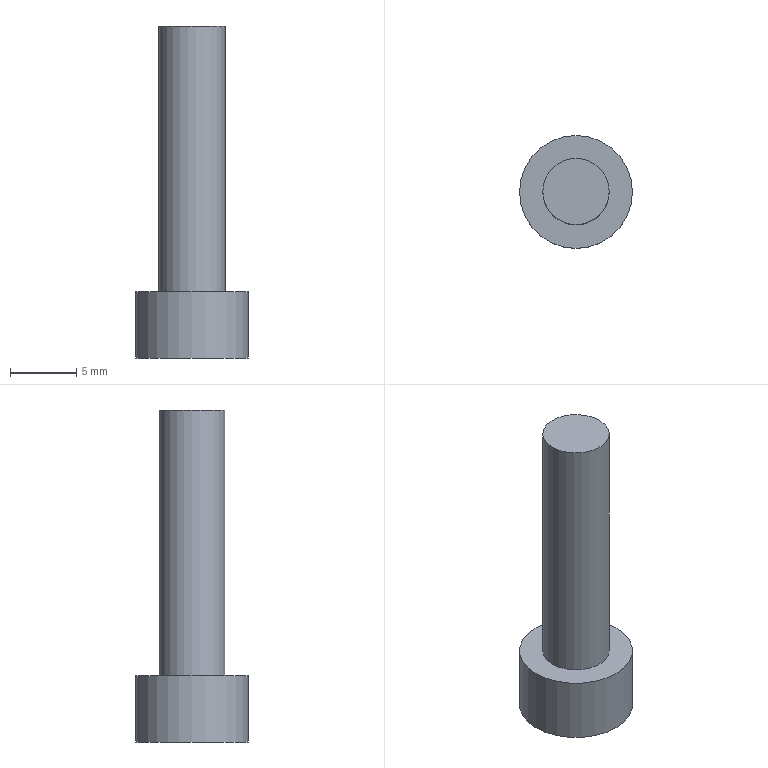Part | STEP file | 1 solid | 12 faces | box 8.5 x 8.5 x 25 mm | volume 630.698 mm3 | plane 10 | cylinder 2 | commonest cylinder face diameters 5 x1 8.5 x1
STEP:
#1=CARTESIAN_POINT('',(0.,0.,0.));
#2=DIRECTION('',(0.,0.,1.));
#3=DIRECTION('',(1.,0.,0.));
#4=AXIS2_PLACEMENT_3D('',#1,#2,#3);
#5=CARTESIAN_POINT('',(1537.233,391.98,-14.081));
#6=VERTEX_POINT('',#5);
#7=CARTESIAN_POINT('',(1541.483,391.98,-14.081));
#8=DIRECTION('',(0.,0.,-1.));
#9=DIRECTION('',(-1.,0.,0.));
#10=AXIS2_PLACEMENT_3D('',#7,#8,#9);
#11=CIRCLE('',#10,4.25);
#12=CARTESIAN_POINT('',(1537.233,391.98,-14.081));
#13=DIRECTION('',(0.,0.,1.));
#14=DIRECTION('',(1.,0.,0.));
#15=AXIS2_PLACEMENT_3D('',#12,#13,#14);
#16=PLANE('',#15);
#17=CARTESIAN_POINT('',(0.,0.));
#18=CARTESIAN_POINT('',(0.,7.361));
#19=CARTESIAN_POINT('',(6.375,3.681));
#20=CARTESIAN_POINT('',(12.75,0.));
#21=CARTESIAN_POINT('',(6.375,-3.681));
#22=CARTESIAN_POINT('',(0.,-7.361));
#23=CARTESIAN_POINT('',(0.,0.));
#24=(BOUNDED_CURVE()B_SPLINE_CURVE(2,(#17,#18,#19,#20,#21,#22,#23),.UNSPECIFIED.,.T.,.F.)B_SPLINE_CURVE_WITH_KNOTS((1,2,2,2,2,1),(-2.094,0.,2.094,4.189,6.283,8.378),.UNSPECIFIED.)CURVE()GEOMETRIC_REPRESENTATION_ITEM()RATIONAL_B_SPLINE_CURVE((1.,0.5,1.,0.5,1.,0.5,1.))REPRESENTATION_ITEM(''));
#25=(GEOMETRIC_REPRESENTATION_CONTEXT(2)PARAMETRIC_REPRESENTATION_CONTEXT()REPRESENTATION_CONTEXT('',''));
#26=DEFINITIONAL_REPRESENTATION('',(#24),#25);
#27=PCURVE('',#16,#26);
#28=CARTESIAN_POINT('',(1541.483,391.98,22.319));
#29=DIRECTION('',(0.,0.,-1.));
#30=DIRECTION('',(-1.,0.,0.));
#31=AXIS2_PLACEMENT_3D('',#28,#29,#30);
#32=CYLINDRICAL_SURFACE('',#31,4.25);
#33=CARTESIAN_POINT('',(0.,36.4));
#34=DIRECTION('',(1.,0.));
#35=VECTOR('',#34,1.);
#36=LINE('',#33,#35);
#37=(GEOMETRIC_REPRESENTATION_CONTEXT(2)PARAMETRIC_REPRESENTATION_CONTEXT()REPRESENTATION_CONTEXT('',''));
#38=DEFINITIONAL_REPRESENTATION('',(#36),#37);
#39=PCURVE('',#32,#38);
#40=SURFACE_CURVE('',#11,(#27,#39),.PCURVE_S1.);
#41=EDGE_CURVE('',#6,#6,#40,.T.);
#42=ORIENTED_EDGE('',*,*,#41,.T.);
#43=EDGE_LOOP('',(#42));
#44=FACE_BOUND('',#43,.T.);
#45=CARTESIAN_POINT('',(1542.638,393.98,-14.081));
#46=VERTEX_POINT('',#45);
#47=CARTESIAN_POINT('',(1540.328,393.98,-14.081));
#48=VERTEX_POINT('',#47);
#49=CARTESIAN_POINT('',(1542.638,393.98,-14.081));
#50=DIRECTION('',(-1.,0.,0.));
#51=VECTOR('',#50,1.);
#52=LINE('',#49,#51);
#53=CARTESIAN_POINT('',(5.405,2.));
#54=DIRECTION('',(-1.,0.));
#55=VECTOR('',#54,1.);
#56=LINE('',#53,#55);
#57=(GEOMETRIC_REPRESENTATION_CONTEXT(2)PARAMETRIC_REPRESENTATION_CONTEXT()REPRESENTATION_CONTEXT('',''));
#58=DEFINITIONAL_REPRESENTATION('',(#56),#57);
#59=PCURVE('',#16,#58);
#60=CARTESIAN_POINT('',(1542.638,393.98,-10.781));
#61=DIRECTION('',(0.,-1.,0.));
#62=DIRECTION('',(-1.,0.,0.));
#63=AXIS2_PLACEMENT_3D('',#60,#61,#62);
#64=PLANE('',#63);
#65=CARTESIAN_POINT('',(0.,3.3));
#66=DIRECTION('',(1.,0.));
#67=VECTOR('',#66,1.);
#68=LINE('',#65,#67);
#69=(GEOMETRIC_REPRESENTATION_CONTEXT(2)PARAMETRIC_REPRESENTATION_CONTEXT()REPRESENTATION_CONTEXT('',''));
#70=DEFINITIONAL_REPRESENTATION('',(#68),#69);
#71=PCURVE('',#64,#70);
#72=SURFACE_CURVE('',#52,(#59,#71),.PCURVE_S1.);
#73=EDGE_CURVE('',#46,#48,#72,.T.);
#74=ORIENTED_EDGE('',*,*,#73,.T.);
#75=CARTESIAN_POINT('',(1539.174,391.98,-14.081));
#76=VERTEX_POINT('',#75);
#77=CARTESIAN_POINT('',(1540.328,393.98,-14.081));
#78=DIRECTION('',(-0.5,-0.866,0.));
#79=VECTOR('',#78,1.);
#80=LINE('',#77,#79);
#81=CARTESIAN_POINT('',(3.095,2.));
#82=DIRECTION('',(-0.5,-0.866));
#83=VECTOR('',#82,1.);
#84=LINE('',#81,#83);
#85=(GEOMETRIC_REPRESENTATION_CONTEXT(2)PARAMETRIC_REPRESENTATION_CONTEXT()REPRESENTATION_CONTEXT('',''));
#86=DEFINITIONAL_REPRESENTATION('',(#84),#85);
#87=PCURVE('',#16,#86);
#88=CARTESIAN_POINT('',(1540.328,393.98,-10.781));
#89=DIRECTION('',(0.866,-0.5,0.));
#90=DIRECTION('',(-0.5,-0.866,0.));
#91=AXIS2_PLACEMENT_3D('',#88,#89,#90);
#92=PLANE('',#91);
#93=CARTESIAN_POINT('',(0.,3.3));
#94=DIRECTION('',(1.,0.));
#95=VECTOR('',#94,1.);
#96=LINE('',#93,#95);
#97=(GEOMETRIC_REPRESENTATION_CONTEXT(2)PARAMETRIC_REPRESENTATION_CONTEXT()REPRESENTATION_CONTEXT('',''));
#98=DEFINITIONAL_REPRESENTATION('',(#96),#97);
#99=PCURVE('',#92,#98);
#100=SURFACE_CURVE('',#80,(#87,#99),.PCURVE_S1.);
#101=EDGE_CURVE('',#48,#76,#100,.T.);
#102=ORIENTED_EDGE('',*,*,#101,.T.);
#103=CARTESIAN_POINT('',(1540.328,389.98,-14.081));
#104=VERTEX_POINT('',#103);
#105=CARTESIAN_POINT('',(1539.174,391.98,-14.081));
#106=DIRECTION('',(0.5,-0.866,0.));
#107=VECTOR('',#106,1.);
#108=LINE('',#105,#107);
#109=CARTESIAN_POINT('',(1.941,0.));
#110=DIRECTION('',(0.5,-0.866));
#111=VECTOR('',#110,1.);
#112=LINE('',#109,#111);
#113=(GEOMETRIC_REPRESENTATION_CONTEXT(2)PARAMETRIC_REPRESENTATION_CONTEXT()REPRESENTATION_CONTEXT('',''));
#114=DEFINITIONAL_REPRESENTATION('',(#112),#113);
#115=PCURVE('',#16,#114);
#116=CARTESIAN_POINT('',(1539.174,391.98,-10.781));
#117=DIRECTION('',(0.866,0.5,0.));
#118=DIRECTION('',(0.5,-0.866,0.));
#119=AXIS2_PLACEMENT_3D('',#116,#117,#118);
#120=PLANE('',#119);
#121=CARTESIAN_POINT('',(0.,3.3));
#122=DIRECTION('',(1.,0.));
#123=VECTOR('',#122,1.);
#124=LINE('',#121,#123);
#125=(GEOMETRIC_REPRESENTATION_CONTEXT(2)PARAMETRIC_REPRESENTATION_CONTEXT()REPRESENTATION_CONTEXT('',''));
#126=DEFINITIONAL_REPRESENTATION('',(#124),#125);
#127=PCURVE('',#120,#126);
#128=SURFACE_CURVE('',#108,(#115,#127),.PCURVE_S1.);
#129=EDGE_CURVE('',#76,#104,#128,.T.);
#130=ORIENTED_EDGE('',*,*,#129,.T.);
#131=CARTESIAN_POINT('',(1542.638,389.98,-14.081));
#132=VERTEX_POINT('',#131);
#133=CARTESIAN_POINT('',(1540.328,389.98,-14.081));
#134=DIRECTION('',(1.,0.,0.));
#135=VECTOR('',#134,1.);
#136=LINE('',#133,#135);
#137=CARTESIAN_POINT('',(3.095,-2.));
#138=DIRECTION('',(1.,0.));
#139=VECTOR('',#138,1.);
#140=LINE('',#137,#139);
#141=(GEOMETRIC_REPRESENTATION_CONTEXT(2)PARAMETRIC_REPRESENTATION_CONTEXT()REPRESENTATION_CONTEXT('',''));
#142=DEFINITIONAL_REPRESENTATION('',(#140),#141);
#143=PCURVE('',#16,#142);
#144=CARTESIAN_POINT('',(1540.328,389.98,-10.781));
#145=DIRECTION('',(0.,1.,0.));
#146=DIRECTION('',(0.,0.,-1.));
#147=AXIS2_PLACEMENT_3D('',#144,#145,#146);
#148=PLANE('',#147);
#149=CARTESIAN_POINT('',(3.3,0.));
#150=DIRECTION('',(0.,-1.));
#151=VECTOR('',#150,1.);
#152=LINE('',#149,#151);
#153=(GEOMETRIC_REPRESENTATION_CONTEXT(2)PARAMETRIC_REPRESENTATION_CONTEXT()REPRESENTATION_CONTEXT('',''));
#154=DEFINITIONAL_REPRESENTATION('',(#152),#153);
#155=PCURVE('',#148,#154);
#156=SURFACE_CURVE('',#136,(#143,#155),.PCURVE_S1.);
#157=EDGE_CURVE('',#104,#132,#156,.T.);
#158=ORIENTED_EDGE('',*,*,#157,.T.);
#159=CARTESIAN_POINT('',(1543.792,391.98,-14.081));
#160=VERTEX_POINT('',#159);
#161=CARTESIAN_POINT('',(1542.638,389.98,-14.081));
#162=DIRECTION('',(0.5,0.866,0.));
#163=VECTOR('',#162,1.);
#164=LINE('',#161,#163);
#165=CARTESIAN_POINT('',(5.405,-2.));
#166=DIRECTION('',(0.5,0.866));
#167=VECTOR('',#166,1.);
#168=LINE('',#165,#167);
#169=(GEOMETRIC_REPRESENTATION_CONTEXT(2)PARAMETRIC_REPRESENTATION_CONTEXT()REPRESENTATION_CONTEXT('',''));
#170=DEFINITIONAL_REPRESENTATION('',(#168),#169);
#171=PCURVE('',#16,#170);
#172=CARTESIAN_POINT('',(1542.638,389.98,-10.781));
#173=DIRECTION('',(-0.866,0.5,0.));
#174=DIRECTION('',(0.5,0.866,0.));
#175=AXIS2_PLACEMENT_3D('',#172,#173,#174);
#176=PLANE('',#175);
#177=CARTESIAN_POINT('',(0.,3.3));
#178=DIRECTION('',(1.,0.));
#179=VECTOR('',#178,1.);
#180=LINE('',#177,#179);
#181=(GEOMETRIC_REPRESENTATION_CONTEXT(2)PARAMETRIC_REPRESENTATION_CONTEXT()REPRESENTATION_CONTEXT('',''));
#182=DEFINITIONAL_REPRESENTATION('',(#180),#181);
#183=PCURVE('',#176,#182);
#184=SURFACE_CURVE('',#164,(#171,#183),.PCURVE_S1.);
#185=EDGE_CURVE('',#132,#160,#184,.T.);
#186=ORIENTED_EDGE('',*,*,#185,.T.);
#187=CARTESIAN_POINT('',(1543.792,391.98,-14.081));
#188=DIRECTION('',(-0.5,0.866,0.));
#189=VECTOR('',#188,1.);
#190=LINE('',#187,#189);
#191=CARTESIAN_POINT('',(6.559,0.));
#192=DIRECTION('',(-0.5,0.866));
#193=VECTOR('',#192,1.);
#194=LINE('',#191,#193);
#195=(GEOMETRIC_REPRESENTATION_CONTEXT(2)PARAMETRIC_REPRESENTATION_CONTEXT()REPRESENTATION_CONTEXT('',''));
#196=DEFINITIONAL_REPRESENTATION('',(#194),#195);
#197=PCURVE('',#16,#196);
#198=CARTESIAN_POINT('',(1543.792,391.98,-10.781));
#199=DIRECTION('',(-0.866,-0.5,0.));
#200=DIRECTION('',(-0.5,0.866,0.));
#201=AXIS2_PLACEMENT_3D('',#198,#199,#200);
#202=PLANE('',#201);
#203=CARTESIAN_POINT('',(0.,3.3));
#204=DIRECTION('',(1.,0.));
#205=VECTOR('',#204,1.);
#206=LINE('',#203,#205);
#207=(GEOMETRIC_REPRESENTATION_CONTEXT(2)PARAMETRIC_REPRESENTATION_CONTEXT()REPRESENTATION_CONTEXT('',''));
#208=DEFINITIONAL_REPRESENTATION('',(#206),#207);
#209=PCURVE('',#202,#208);
#210=SURFACE_CURVE('',#190,(#197,#209),.PCURVE_S1.);
#211=EDGE_CURVE('',#160,#46,#210,.T.);
#212=ORIENTED_EDGE('',*,*,#211,.T.);
#213=EDGE_LOOP('',(#74,#102,#130,#158,#186,#212));
#214=FACE_BOUND('',#213,.T.);
#215=ADVANCED_FACE('',(#44,#214),#16,.F.);
#216=ORIENTED_EDGE('',*,*,#41,.F.);
#217=CARTESIAN_POINT('',(1537.233,391.98,-9.081));
#218=VERTEX_POINT('',#217);
#219=CARTESIAN_POINT('',(1537.233,391.98,-9.081));
#220=CARTESIAN_POINT('',(1537.233,391.98,-14.081));
#221=B_SPLINE_CURVE_WITH_KNOTS('',1,(#219,#220),.UNSPECIFIED.,.F.,.F.,(2,2),(31.4,36.4),.PIECEWISE_BEZIER_KNOTS.);
#222=CARTESIAN_POINT('',(0.,0.));
#223=DIRECTION('',(0.,1.));
#224=VECTOR('',#223,1.);
#225=LINE('',#222,#224);
#226=(GEOMETRIC_REPRESENTATION_CONTEXT(2)PARAMETRIC_REPRESENTATION_CONTEXT()REPRESENTATION_CONTEXT('',''));
#227=DEFINITIONAL_REPRESENTATION('',(#225),#226);
#228=PCURVE('',#32,#227);
#229=CARTESIAN_POINT('',(6.283,0.));
#230=DIRECTION('',(0.,1.));
#231=VECTOR('',#230,1.);
#232=LINE('',#229,#231);
#233=(GEOMETRIC_REPRESENTATION_CONTEXT(2)PARAMETRIC_REPRESENTATION_CONTEXT()REPRESENTATION_CONTEXT('',''));
#234=DEFINITIONAL_REPRESENTATION('',(#232),#233);
#235=PCURVE('',#32,#234);
#236=SEAM_CURVE('',#221,(#228,#235),.PCURVE_S1.);
#237=EDGE_CURVE('',#218,#6,#236,.T.);
#238=ORIENTED_EDGE('',*,*,#237,.F.);
#239=CARTESIAN_POINT('',(1541.483,391.98,-9.081));
#240=DIRECTION('',(0.,0.,-1.));
#241=DIRECTION('',(-1.,0.,0.));
#242=AXIS2_PLACEMENT_3D('',#239,#240,#241);
#243=CIRCLE('',#242,4.25);
#244=CARTESIAN_POINT('',(0.,31.4));
#245=DIRECTION('',(1.,0.));
#246=VECTOR('',#245,1.);
#247=LINE('',#244,#246);
#248=(GEOMETRIC_REPRESENTATION_CONTEXT(2)PARAMETRIC_REPRESENTATION_CONTEXT()REPRESENTATION_CONTEXT('',''));
#249=DEFINITIONAL_REPRESENTATION('',(#247),#248);
#250=PCURVE('',#32,#249);
#251=CARTESIAN_POINT('',(1538.983,391.98,-9.081));
#252=DIRECTION('',(0.,0.,-1.));
#253=DIRECTION('',(-1.,0.,0.));
#254=AXIS2_PLACEMENT_3D('',#251,#252,#253);
#255=PLANE('',#254);
#256=CARTESIAN_POINT('',(-2.5,0.));
#257=DIRECTION('',(1.,0.));
#258=AXIS2_PLACEMENT_2D('',#256,#257);
#259=CIRCLE('',#258,4.25);
#260=(GEOMETRIC_REPRESENTATION_CONTEXT(2)PARAMETRIC_REPRESENTATION_CONTEXT()REPRESENTATION_CONTEXT('',''));
#261=DEFINITIONAL_REPRESENTATION('',(#259),#260);
#262=PCURVE('',#255,#261);
#263=SURFACE_CURVE('',#243,(#250,#262),.PCURVE_S1.);
#264=EDGE_CURVE('',#218,#218,#263,.T.);
#265=ORIENTED_EDGE('',*,*,#264,.T.);
#266=ORIENTED_EDGE('',*,*,#237,.T.);
#267=EDGE_LOOP('',(#216,#238,#265,#266));
#268=FACE_BOUND('',#267,.T.);
#269=ADVANCED_FACE('',(#268),#32,.T.);
#270=ORIENTED_EDGE('',*,*,#264,.F.);
#271=EDGE_LOOP('',(#270));
#272=FACE_BOUND('',#271,.T.);
#273=CARTESIAN_POINT('',(1538.983,391.98,-9.081));
#274=VERTEX_POINT('',#273);
#275=CARTESIAN_POINT('',(1541.483,391.98,-9.081));
#276=DIRECTION('',(0.,0.,-1.));
#277=DIRECTION('',(-1.,0.,0.));
#278=AXIS2_PLACEMENT_3D('',#275,#276,#277);
#279=CIRCLE('',#278,2.5);
#280=CARTESIAN_POINT('',(-2.5,0.));
#281=DIRECTION('',(1.,0.));
#282=AXIS2_PLACEMENT_2D('',#280,#281);
#283=CIRCLE('',#282,2.5);
#284=(GEOMETRIC_REPRESENTATION_CONTEXT(2)PARAMETRIC_REPRESENTATION_CONTEXT()REPRESENTATION_CONTEXT('',''));
#285=DEFINITIONAL_REPRESENTATION('',(#283),#284);
#286=PCURVE('',#255,#285);
#287=CARTESIAN_POINT('',(1541.483,391.98,22.319));
#288=DIRECTION('',(0.,0.,-1.));
#289=DIRECTION('',(-1.,0.,0.));
#290=AXIS2_PLACEMENT_3D('',#287,#288,#289);
#291=CYLINDRICAL_SURFACE('',#290,2.5);
#292=CARTESIAN_POINT('',(0.,31.4));
#293=DIRECTION('',(1.,0.));
#294=VECTOR('',#293,1.);
#295=LINE('',#292,#294);
#296=(GEOMETRIC_REPRESENTATION_CONTEXT(2)PARAMETRIC_REPRESENTATION_CONTEXT()REPRESENTATION_CONTEXT('',''));
#297=DEFINITIONAL_REPRESENTATION('',(#295),#296);
#298=PCURVE('',#291,#297);
#299=SURFACE_CURVE('',#279,(#286,#298),.PCURVE_S1.);
#300=EDGE_CURVE('',#274,#274,#299,.T.);
#301=ORIENTED_EDGE('',*,*,#300,.T.);
#302=EDGE_LOOP('',(#301));
#303=FACE_BOUND('',#302,.T.);
#304=ADVANCED_FACE('',(#272,#303),#255,.F.);
#305=ORIENTED_EDGE('',*,*,#300,.F.);
#306=CARTESIAN_POINT('',(1538.983,391.98,10.919));
#307=VERTEX_POINT('',#306);
#308=CARTESIAN_POINT('',(1538.983,391.98,10.919));
#309=CARTESIAN_POINT('',(1538.983,391.98,-9.081));
#310=B_SPLINE_CURVE_WITH_KNOTS('',1,(#308,#309),.UNSPECIFIED.,.F.,.F.,(2,2),(11.4,31.4),.PIECEWISE_BEZIER_KNOTS.);
#311=CARTESIAN_POINT('',(0.,0.));
#312=DIRECTION('',(0.,1.));
#313=VECTOR('',#312,1.);
#314=LINE('',#311,#313);
#315=(GEOMETRIC_REPRESENTATION_CONTEXT(2)PARAMETRIC_REPRESENTATION_CONTEXT()REPRESENTATION_CONTEXT('',''));
#316=DEFINITIONAL_REPRESENTATION('',(#314),#315);
#317=PCURVE('',#291,#316);
#318=CARTESIAN_POINT('',(6.283,0.));
#319=DIRECTION('',(0.,1.));
#320=VECTOR('',#319,1.);
#321=LINE('',#318,#320);
#322=(GEOMETRIC_REPRESENTATION_CONTEXT(2)PARAMETRIC_REPRESENTATION_CONTEXT()REPRESENTATION_CONTEXT('',''));
#323=DEFINITIONAL_REPRESENTATION('',(#321),#322);
#324=PCURVE('',#291,#323);
#325=SEAM_CURVE('',#310,(#317,#324),.PCURVE_S1.);
#326=EDGE_CURVE('',#307,#274,#325,.T.);
#327=ORIENTED_EDGE('',*,*,#326,.F.);
#328=CARTESIAN_POINT('',(1541.483,391.98,10.919));
#329=DIRECTION('',(0.,0.,-1.));
#330=DIRECTION('',(-1.,0.,0.));
#331=AXIS2_PLACEMENT_3D('',#328,#329,#330);
#332=CIRCLE('',#331,2.5);
#333=CARTESIAN_POINT('',(0.,11.4));
#334=DIRECTION('',(1.,0.));
#335=VECTOR('',#334,1.);
#336=LINE('',#333,#335);
#337=(GEOMETRIC_REPRESENTATION_CONTEXT(2)PARAMETRIC_REPRESENTATION_CONTEXT()REPRESENTATION_CONTEXT('',''));
#338=DEFINITIONAL_REPRESENTATION('',(#336),#337);
#339=PCURVE('',#291,#338);
#340=CARTESIAN_POINT('',(1541.483,391.98,10.919));
#341=DIRECTION('',(0.,0.,-1.));
#342=DIRECTION('',(-1.,0.,0.));
#343=AXIS2_PLACEMENT_3D('',#340,#341,#342);
#344=PLANE('',#343);
#345=CARTESIAN_POINT('',(0.,0.));
#346=DIRECTION('',(1.,0.));
#347=AXIS2_PLACEMENT_2D('',#345,#346);
#348=CIRCLE('',#347,2.5);
#349=(GEOMETRIC_REPRESENTATION_CONTEXT(2)PARAMETRIC_REPRESENTATION_CONTEXT()REPRESENTATION_CONTEXT('',''));
#350=DEFINITIONAL_REPRESENTATION('',(#348),#349);
#351=PCURVE('',#344,#350);
#352=SURFACE_CURVE('',#332,(#339,#351),.PCURVE_S1.);
#353=EDGE_CURVE('',#307,#307,#352,.T.);
#354=ORIENTED_EDGE('',*,*,#353,.T.);
#355=ORIENTED_EDGE('',*,*,#326,.T.);
#356=EDGE_LOOP('',(#305,#327,#354,#355));
#357=FACE_BOUND('',#356,.T.);
#358=ADVANCED_FACE('',(#357),#291,.T.);
#359=ORIENTED_EDGE('',*,*,#353,.F.);
#360=EDGE_LOOP('',(#359));
#361=FACE_BOUND('',#360,.T.);
#362=ADVANCED_FACE('',(#361),#344,.F.);
#363=ORIENTED_EDGE('',*,*,#73,.F.);
#364=CARTESIAN_POINT('',(1542.638,393.98,-10.781));
#365=VERTEX_POINT('',#364);
#366=CARTESIAN_POINT('',(1542.638,393.98,-10.781));
#367=DIRECTION('',(0.,0.,1.));
#368=VECTOR('',#367,1.);
#369=LINE('',#366,#368);
#370=CARTESIAN_POINT('',(0.,0.));
#371=DIRECTION('',(0.,-1.));
#372=VECTOR('',#371,1.);
#373=LINE('',#370,#372);
#374=(GEOMETRIC_REPRESENTATION_CONTEXT(2)PARAMETRIC_REPRESENTATION_CONTEXT()REPRESENTATION_CONTEXT('',''));
#375=DEFINITIONAL_REPRESENTATION('',(#373),#374);
#376=PCURVE('',#64,#375);
#377=CARTESIAN_POINT('',(2.309,0.));
#378=DIRECTION('',(0.,-1.));
#379=VECTOR('',#378,1.);
#380=LINE('',#377,#379);
#381=(GEOMETRIC_REPRESENTATION_CONTEXT(2)PARAMETRIC_REPRESENTATION_CONTEXT()REPRESENTATION_CONTEXT('',''));
#382=DEFINITIONAL_REPRESENTATION('',(#380),#381);
#383=PCURVE('',#202,#382);
#384=SURFACE_CURVE('',#369,(#376,#383),.PCURVE_S1.);
#385=EDGE_CURVE('',#46,#365,#384,.T.);
#386=ORIENTED_EDGE('',*,*,#385,.T.);
#387=CARTESIAN_POINT('',(1540.328,393.98,-10.781));
#388=VERTEX_POINT('',#387);
#389=CARTESIAN_POINT('',(1542.638,393.98,-10.781));
#390=DIRECTION('',(1.,0.,0.));
#391=VECTOR('',#390,1.);
#392=LINE('',#389,#391);
#393=CARTESIAN_POINT('',(0.,0.));
#394=DIRECTION('',(-1.,0.));
#395=VECTOR('',#394,1.);
#396=LINE('',#393,#395);
#397=(GEOMETRIC_REPRESENTATION_CONTEXT(2)PARAMETRIC_REPRESENTATION_CONTEXT()REPRESENTATION_CONTEXT('',''));
#398=DEFINITIONAL_REPRESENTATION('',(#396),#397);
#399=PCURVE('',#64,#398);
#400=CARTESIAN_POINT('',(1541.483,391.98,-10.781));
#401=DIRECTION('',(0.,0.,1.));
#402=DIRECTION('',(1.,0.,0.));
#403=AXIS2_PLACEMENT_3D('',#400,#401,#402);
#404=PLANE('',#403);
#405=CARTESIAN_POINT('',(1.155,2.));
#406=DIRECTION('',(1.,0.));
#407=VECTOR('',#406,1.);
#408=LINE('',#405,#407);
#409=(GEOMETRIC_REPRESENTATION_CONTEXT(2)PARAMETRIC_REPRESENTATION_CONTEXT()REPRESENTATION_CONTEXT('',''));
#410=DEFINITIONAL_REPRESENTATION('',(#408),#409);
#411=PCURVE('',#404,#410);
#412=SURFACE_CURVE('',#392,(#399,#411),.PCURVE_S1.);
#413=EDGE_CURVE('',#388,#365,#412,.T.);
#414=ORIENTED_EDGE('',*,*,#413,.F.);
#415=CARTESIAN_POINT('',(1540.328,393.98,-10.781));
#416=DIRECTION('',(0.,0.,1.));
#417=VECTOR('',#416,1.);
#418=LINE('',#415,#417);
#419=CARTESIAN_POINT('',(2.309,0.));
#420=DIRECTION('',(0.,-1.));
#421=VECTOR('',#420,1.);
#422=LINE('',#419,#421);
#423=(GEOMETRIC_REPRESENTATION_CONTEXT(2)PARAMETRIC_REPRESENTATION_CONTEXT()REPRESENTATION_CONTEXT('',''));
#424=DEFINITIONAL_REPRESENTATION('',(#422),#423);
#425=PCURVE('',#64,#424);
#426=CARTESIAN_POINT('',(0.,0.));
#427=DIRECTION('',(0.,-1.));
#428=VECTOR('',#427,1.);
#429=LINE('',#426,#428);
#430=(GEOMETRIC_REPRESENTATION_CONTEXT(2)PARAMETRIC_REPRESENTATION_CONTEXT()REPRESENTATION_CONTEXT('',''));
#431=DEFINITIONAL_REPRESENTATION('',(#429),#430);
#432=PCURVE('',#92,#431);
#433=SURFACE_CURVE('',#418,(#425,#432),.PCURVE_S1.);
#434=EDGE_CURVE('',#48,#388,#433,.T.);
#435=ORIENTED_EDGE('',*,*,#434,.F.);
#436=EDGE_LOOP('',(#363,#386,#414,#435));
#437=FACE_BOUND('',#436,.T.);
#438=ADVANCED_FACE('',(#437),#64,.T.);
#439=ORIENTED_EDGE('',*,*,#101,.F.);
#440=ORIENTED_EDGE('',*,*,#434,.T.);
#441=CARTESIAN_POINT('',(1539.174,391.98,-10.781));
#442=VERTEX_POINT('',#441);
#443=CARTESIAN_POINT('',(1540.328,393.98,-10.781));
#444=DIRECTION('',(0.5,0.866,0.));
#445=VECTOR('',#444,1.);
#446=LINE('',#443,#445);
#447=CARTESIAN_POINT('',(0.,0.));
#448=DIRECTION('',(-1.,0.));
#449=VECTOR('',#448,1.);
#450=LINE('',#447,#449);
#451=(GEOMETRIC_REPRESENTATION_CONTEXT(2)PARAMETRIC_REPRESENTATION_CONTEXT()REPRESENTATION_CONTEXT('',''));
#452=DEFINITIONAL_REPRESENTATION('',(#450),#451);
#453=PCURVE('',#92,#452);
#454=CARTESIAN_POINT('',(-1.155,2.));
#455=DIRECTION('',(0.5,0.866));
#456=VECTOR('',#455,1.);
#457=LINE('',#454,#456);
#458=(GEOMETRIC_REPRESENTATION_CONTEXT(2)PARAMETRIC_REPRESENTATION_CONTEXT()REPRESENTATION_CONTEXT('',''));
#459=DEFINITIONAL_REPRESENTATION('',(#457),#458);
#460=PCURVE('',#404,#459);
#461=SURFACE_CURVE('',#446,(#453,#460),.PCURVE_S1.);
#462=EDGE_CURVE('',#442,#388,#461,.T.);
#463=ORIENTED_EDGE('',*,*,#462,.F.);
#464=CARTESIAN_POINT('',(1539.174,391.98,-10.781));
#465=DIRECTION('',(0.,0.,1.));
#466=VECTOR('',#465,1.);
#467=LINE('',#464,#466);
#468=CARTESIAN_POINT('',(2.309,0.));
#469=DIRECTION('',(0.,-1.));
#470=VECTOR('',#469,1.);
#471=LINE('',#468,#470);
#472=(GEOMETRIC_REPRESENTATION_CONTEXT(2)PARAMETRIC_REPRESENTATION_CONTEXT()REPRESENTATION_CONTEXT('',''));
#473=DEFINITIONAL_REPRESENTATION('',(#471),#472);
#474=PCURVE('',#92,#473);
#475=CARTESIAN_POINT('',(0.,0.));
#476=DIRECTION('',(0.,-1.));
#477=VECTOR('',#476,1.);
#478=LINE('',#475,#477);
#479=(GEOMETRIC_REPRESENTATION_CONTEXT(2)PARAMETRIC_REPRESENTATION_CONTEXT()REPRESENTATION_CONTEXT('',''));
#480=DEFINITIONAL_REPRESENTATION('',(#478),#479);
#481=PCURVE('',#120,#480);
#482=SURFACE_CURVE('',#467,(#474,#481),.PCURVE_S1.);
#483=EDGE_CURVE('',#76,#442,#482,.T.);
#484=ORIENTED_EDGE('',*,*,#483,.F.);
#485=EDGE_LOOP('',(#439,#440,#463,#484));
#486=FACE_BOUND('',#485,.T.);
#487=ADVANCED_FACE('',(#486),#92,.T.);
#488=ORIENTED_EDGE('',*,*,#129,.F.);
#489=ORIENTED_EDGE('',*,*,#483,.T.);
#490=CARTESIAN_POINT('',(1540.328,389.98,-10.781));
#491=VERTEX_POINT('',#490);
#492=CARTESIAN_POINT('',(1539.174,391.98,-10.781));
#493=DIRECTION('',(-0.5,0.866,0.));
#494=VECTOR('',#493,1.);
#495=LINE('',#492,#494);
#496=CARTESIAN_POINT('',(0.,0.));
#497=DIRECTION('',(-1.,0.));
#498=VECTOR('',#497,1.);
#499=LINE('',#496,#498);
#500=(GEOMETRIC_REPRESENTATION_CONTEXT(2)PARAMETRIC_REPRESENTATION_CONTEXT()REPRESENTATION_CONTEXT('',''));
#501=DEFINITIONAL_REPRESENTATION('',(#499),#500);
#502=PCURVE('',#120,#501);
#503=CARTESIAN_POINT('',(-2.309,0.));
#504=DIRECTION('',(-0.5,0.866));
#505=VECTOR('',#504,1.);
#506=LINE('',#503,#505);
#507=(GEOMETRIC_REPRESENTATION_CONTEXT(2)PARAMETRIC_REPRESENTATION_CONTEXT()REPRESENTATION_CONTEXT('',''));
#508=DEFINITIONAL_REPRESENTATION('',(#506),#507);
#509=PCURVE('',#404,#508);
#510=SURFACE_CURVE('',#495,(#502,#509),.PCURVE_S1.);
#511=EDGE_CURVE('',#491,#442,#510,.T.);
#512=ORIENTED_EDGE('',*,*,#511,.F.);
#513=CARTESIAN_POINT('',(1540.328,389.98,-10.781));
#514=DIRECTION('',(0.,0.,1.));
#515=VECTOR('',#514,1.);
#516=LINE('',#513,#515);
#517=CARTESIAN_POINT('',(2.309,0.));
#518=DIRECTION('',(0.,-1.));
#519=VECTOR('',#518,1.);
#520=LINE('',#517,#519);
#521=(GEOMETRIC_REPRESENTATION_CONTEXT(2)PARAMETRIC_REPRESENTATION_CONTEXT()REPRESENTATION_CONTEXT('',''));
#522=DEFINITIONAL_REPRESENTATION('',(#520),#521);
#523=PCURVE('',#120,#522);
#524=CARTESIAN_POINT('',(0.,0.));
#525=DIRECTION('',(-1.,0.));
#526=VECTOR('',#525,1.);
#527=LINE('',#524,#526);
#528=(GEOMETRIC_REPRESENTATION_CONTEXT(2)PARAMETRIC_REPRESENTATION_CONTEXT()REPRESENTATION_CONTEXT('',''));
#529=DEFINITIONAL_REPRESENTATION('',(#527),#528);
#530=PCURVE('',#148,#529);
#531=SURFACE_CURVE('',#516,(#523,#530),.PCURVE_S1.);
#532=EDGE_CURVE('',#104,#491,#531,.T.);
#533=ORIENTED_EDGE('',*,*,#532,.F.);
#534=EDGE_LOOP('',(#488,#489,#512,#533));
#535=FACE_BOUND('',#534,.T.);
#536=ADVANCED_FACE('',(#535),#120,.T.);
#537=ORIENTED_EDGE('',*,*,#157,.F.);
#538=ORIENTED_EDGE('',*,*,#532,.T.);
#539=CARTESIAN_POINT('',(1542.638,389.98,-10.781));
#540=VERTEX_POINT('',#539);
#541=CARTESIAN_POINT('',(1540.328,389.98,-10.781));
#542=DIRECTION('',(-1.,0.,0.));
#543=VECTOR('',#542,1.);
#544=LINE('',#541,#543);
#545=CARTESIAN_POINT('',(0.,0.));
#546=DIRECTION('',(0.,1.));
#547=VECTOR('',#546,1.);
#548=LINE('',#545,#547);
#549=(GEOMETRIC_REPRESENTATION_CONTEXT(2)PARAMETRIC_REPRESENTATION_CONTEXT()REPRESENTATION_CONTEXT('',''));
#550=DEFINITIONAL_REPRESENTATION('',(#548),#549);
#551=PCURVE('',#148,#550);
#552=CARTESIAN_POINT('',(-1.155,-2.));
#553=DIRECTION('',(-1.,0.));
#554=VECTOR('',#553,1.);
#555=LINE('',#552,#554);
#556=(GEOMETRIC_REPRESENTATION_CONTEXT(2)PARAMETRIC_REPRESENTATION_CONTEXT()REPRESENTATION_CONTEXT('',''));
#557=DEFINITIONAL_REPRESENTATION('',(#555),#556);
#558=PCURVE('',#404,#557);
#559=SURFACE_CURVE('',#544,(#551,#558),.PCURVE_S1.);
#560=EDGE_CURVE('',#540,#491,#559,.T.);
#561=ORIENTED_EDGE('',*,*,#560,.F.);
#562=CARTESIAN_POINT('',(1542.638,389.98,-10.781));
#563=DIRECTION('',(0.,0.,1.));
#564=VECTOR('',#563,1.);
#565=LINE('',#562,#564);
#566=CARTESIAN_POINT('',(0.,-2.309));
#567=DIRECTION('',(-1.,0.));
#568=VECTOR('',#567,1.);
#569=LINE('',#566,#568);
#570=(GEOMETRIC_REPRESENTATION_CONTEXT(2)PARAMETRIC_REPRESENTATION_CONTEXT()REPRESENTATION_CONTEXT('',''));
#571=DEFINITIONAL_REPRESENTATION('',(#569),#570);
#572=PCURVE('',#148,#571);
#573=CARTESIAN_POINT('',(0.,0.));
#574=DIRECTION('',(0.,-1.));
#575=VECTOR('',#574,1.);
#576=LINE('',#573,#575);
#577=(GEOMETRIC_REPRESENTATION_CONTEXT(2)PARAMETRIC_REPRESENTATION_CONTEXT()REPRESENTATION_CONTEXT('',''));
#578=DEFINITIONAL_REPRESENTATION('',(#576),#577);
#579=PCURVE('',#176,#578);
#580=SURFACE_CURVE('',#565,(#572,#579),.PCURVE_S1.);
#581=EDGE_CURVE('',#132,#540,#580,.T.);
#582=ORIENTED_EDGE('',*,*,#581,.F.);
#583=EDGE_LOOP('',(#537,#538,#561,#582));
#584=FACE_BOUND('',#583,.T.);
#585=ADVANCED_FACE('',(#584),#148,.T.);
#586=ORIENTED_EDGE('',*,*,#185,.F.);
#587=ORIENTED_EDGE('',*,*,#581,.T.);
#588=CARTESIAN_POINT('',(1543.792,391.98,-10.781));
#589=VERTEX_POINT('',#588);
#590=CARTESIAN_POINT('',(1542.638,389.98,-10.781));
#591=DIRECTION('',(-0.5,-0.866,0.));
#592=VECTOR('',#591,1.);
#593=LINE('',#590,#592);
#594=CARTESIAN_POINT('',(0.,0.));
#595=DIRECTION('',(-1.,0.));
#596=VECTOR('',#595,1.);
#597=LINE('',#594,#596);
#598=(GEOMETRIC_REPRESENTATION_CONTEXT(2)PARAMETRIC_REPRESENTATION_CONTEXT()REPRESENTATION_CONTEXT('',''));
#599=DEFINITIONAL_REPRESENTATION('',(#597),#598);
#600=PCURVE('',#176,#599);
#601=CARTESIAN_POINT('',(1.155,-2.));
#602=DIRECTION('',(-0.5,-0.866));
#603=VECTOR('',#602,1.);
#604=LINE('',#601,#603);
#605=(GEOMETRIC_REPRESENTATION_CONTEXT(2)PARAMETRIC_REPRESENTATION_CONTEXT()REPRESENTATION_CONTEXT('',''));
#606=DEFINITIONAL_REPRESENTATION('',(#604),#605);
#607=PCURVE('',#404,#606);
#608=SURFACE_CURVE('',#593,(#600,#607),.PCURVE_S1.);
#609=EDGE_CURVE('',#589,#540,#608,.T.);
#610=ORIENTED_EDGE('',*,*,#609,.F.);
#611=CARTESIAN_POINT('',(1543.792,391.98,-10.781));
#612=DIRECTION('',(0.,0.,1.));
#613=VECTOR('',#612,1.);
#614=LINE('',#611,#613);
#615=CARTESIAN_POINT('',(2.309,0.));
#616=DIRECTION('',(0.,-1.));
#617=VECTOR('',#616,1.);
#618=LINE('',#615,#617);
#619=(GEOMETRIC_REPRESENTATION_CONTEXT(2)PARAMETRIC_REPRESENTATION_CONTEXT()REPRESENTATION_CONTEXT('',''));
#620=DEFINITIONAL_REPRESENTATION('',(#618),#619);
#621=PCURVE('',#176,#620);
#622=CARTESIAN_POINT('',(0.,0.));
#623=DIRECTION('',(0.,-1.));
#624=VECTOR('',#623,1.);
#625=LINE('',#622,#624);
#626=(GEOMETRIC_REPRESENTATION_CONTEXT(2)PARAMETRIC_REPRESENTATION_CONTEXT()REPRESENTATION_CONTEXT('',''));
#627=DEFINITIONAL_REPRESENTATION('',(#625),#626);
#628=PCURVE('',#202,#627);
#629=SURFACE_CURVE('',#614,(#621,#628),.PCURVE_S1.);
#630=EDGE_CURVE('',#160,#589,#629,.T.);
#631=ORIENTED_EDGE('',*,*,#630,.F.);
#632=EDGE_LOOP('',(#586,#587,#610,#631));
#633=FACE_BOUND('',#632,.T.);
#634=ADVANCED_FACE('',(#633),#176,.T.);
#635=ORIENTED_EDGE('',*,*,#211,.F.);
#636=ORIENTED_EDGE('',*,*,#630,.T.);
#637=CARTESIAN_POINT('',(1543.792,391.98,-10.781));
#638=DIRECTION('',(0.5,-0.866,0.));
#639=VECTOR('',#638,1.);
#640=LINE('',#637,#639);
#641=CARTESIAN_POINT('',(0.,0.));
#642=DIRECTION('',(-1.,0.));
#643=VECTOR('',#642,1.);
#644=LINE('',#641,#643);
#645=(GEOMETRIC_REPRESENTATION_CONTEXT(2)PARAMETRIC_REPRESENTATION_CONTEXT()REPRESENTATION_CONTEXT('',''));
#646=DEFINITIONAL_REPRESENTATION('',(#644),#645);
#647=PCURVE('',#202,#646);
#648=CARTESIAN_POINT('',(2.309,0.));
#649=DIRECTION('',(0.5,-0.866));
#650=VECTOR('',#649,1.);
#651=LINE('',#648,#650);
#652=(GEOMETRIC_REPRESENTATION_CONTEXT(2)PARAMETRIC_REPRESENTATION_CONTEXT()REPRESENTATION_CONTEXT('',''));
#653=DEFINITIONAL_REPRESENTATION('',(#651),#652);
#654=PCURVE('',#404,#653);
#655=SURFACE_CURVE('',#640,(#647,#654),.PCURVE_S1.);
#656=EDGE_CURVE('',#365,#589,#655,.T.);
#657=ORIENTED_EDGE('',*,*,#656,.F.);
#658=ORIENTED_EDGE('',*,*,#385,.F.);
#659=EDGE_LOOP('',(#635,#636,#657,#658));
#660=FACE_BOUND('',#659,.T.);
#661=ADVANCED_FACE('',(#660),#202,.T.);
#662=ORIENTED_EDGE('',*,*,#413,.T.);
#663=ORIENTED_EDGE('',*,*,#656,.T.);
#664=ORIENTED_EDGE('',*,*,#609,.T.);
#665=ORIENTED_EDGE('',*,*,#560,.T.);
#666=ORIENTED_EDGE('',*,*,#511,.T.);
#667=ORIENTED_EDGE('',*,*,#462,.T.);
#668=EDGE_LOOP('',(#662,#663,#664,#665,#666,#667));
#669=FACE_BOUND('',#668,.T.);
#670=ADVANCED_FACE('',(#669),#404,.F.);
#671=CLOSED_SHELL('',(#215,#269,#304,#358,#362,#438,#487,#536,#585,#634,#661,#670));
#672=MANIFOLD_SOLID_BREP('',#671);
#673=(LENGTH_UNIT()NAMED_UNIT(*)SI_UNIT(.MILLI.,.METRE.));
#674=UNCERTAINTY_MEASURE_WITH_UNIT(LENGTH_MEASURE(0.000002),#673,'','');
#675=(NAMED_UNIT(*)PLANE_ANGLE_UNIT()SI_UNIT($,.RADIAN.));
#676=(NAMED_UNIT(*)SI_UNIT($,.STERADIAN.)SOLID_ANGLE_UNIT());
#677=(GEOMETRIC_REPRESENTATION_CONTEXT(3)GLOBAL_UNCERTAINTY_ASSIGNED_CONTEXT((#674))GLOBAL_UNIT_ASSIGNED_CONTEXT((#673,#675,#676))REPRESENTATION_CONTEXT('',''));
#678=ADVANCED_BREP_SHAPE_REPRESENTATION('',(#4,#672),#677);